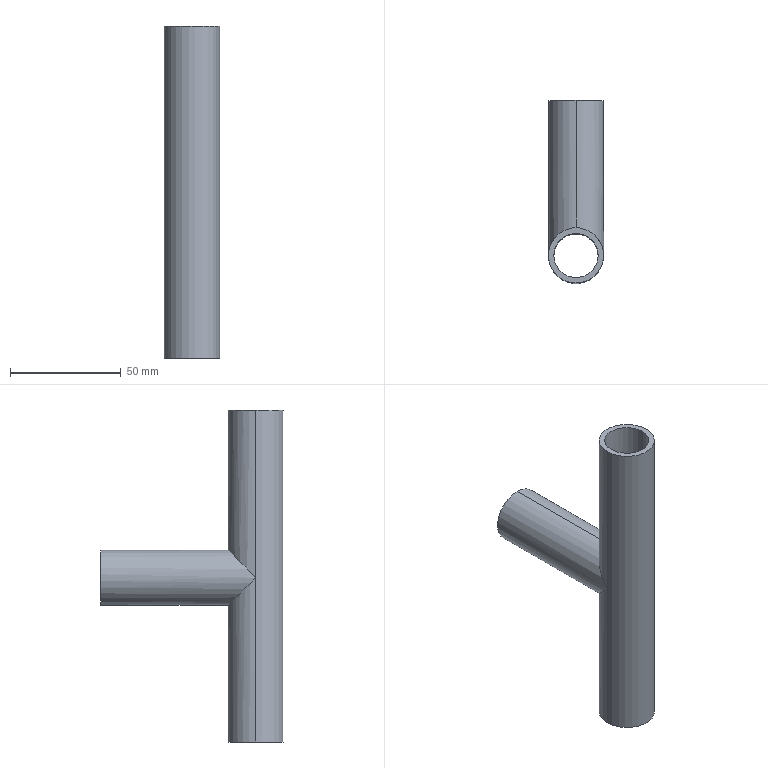Part | SolidWorks | features ICE 2, BaseBody 1 | 1 solid | 17 faces | box 25 x 82.626 x 150 mm | volume 36350 mm3 | cylinder 12 | plane 5 | commonest cylinder face diameters 20 x7 25 x5
STEP:
#1=CARTESIAN_POINT('',(0.,10.,64.222));
#2=VERTEX_POINT('',#1);
#3=CARTESIAN_POINT('',(-10.,0.,74.222));
#4=VERTEX_POINT('',#3);
#5=CARTESIAN_POINT('',(0.,10.,64.222));
#6=CARTESIAN_POINT('',(-5.858,10.,64.222));
#7=CARTESIAN_POINT('',(-10.,5.858,68.365));
#8=CARTESIAN_POINT('',(-10.,0.,74.222));
#9=(BOUNDED_CURVE()B_SPLINE_CURVE(3,(#5,#6,#7,#8),.UNSPECIFIED.,.F.,.F.)B_SPLINE_CURVE_WITH_KNOTS((4,4),(0.,1.571),.UNSPECIFIED.)CURVE()GEOMETRIC_REPRESENTATION_ITEM()RATIONAL_B_SPLINE_CURVE((1.,0.8047,0.8047,1.))REPRESENTATION_ITEM(''));
#10=EDGE_CURVE('',#2,#4,#9,.T.);
#11=ORIENTED_EDGE('',*,*,#10,.F.);
#12=CARTESIAN_POINT('',(0.,70.126,64.222));
#13=VERTEX_POINT('',#12);
#14=CARTESIAN_POINT('',(0.,-3.874,64.222));
#15=DIRECTION('',(0.,1.,0.));
#16=VECTOR('',#15,1000.);
#17=LINE('',#14,#16);
#18=EDGE_CURVE('',#2,#13,#17,.T.);
#19=ORIENTED_EDGE('',*,*,#18,.T.);
#20=CARTESIAN_POINT('',(0.,70.126,84.222));
#21=VERTEX_POINT('',#20);
#22=CARTESIAN_POINT('',(0.,70.126,74.222));
#23=DIRECTION('',(0.,1.,0.));
#24=DIRECTION('',(0.,0.,1.));
#25=AXIS2_PLACEMENT_3D('',#22,#23,#24);
#26=CIRCLE('',#25,10.);
#27=EDGE_CURVE('',#13,#21,#26,.T.);
#28=ORIENTED_EDGE('',*,*,#27,.T.);
#29=CARTESIAN_POINT('',(0.,10.,84.222));
#30=VERTEX_POINT('',#29);
#31=CARTESIAN_POINT('',(0.,-3.874,84.222));
#32=DIRECTION('',(0.,1.,0.));
#33=VECTOR('',#32,1000.);
#34=LINE('',#31,#33);
#35=EDGE_CURVE('',#30,#21,#34,.T.);
#36=ORIENTED_EDGE('',*,*,#35,.F.);
#37=CARTESIAN_POINT('',(-10.,0.,74.222));
#38=CARTESIAN_POINT('',(-10.,5.858,80.08));
#39=CARTESIAN_POINT('',(-5.858,10.,84.222));
#40=CARTESIAN_POINT('',(0.,10.,84.222));
#41=(BOUNDED_CURVE()B_SPLINE_CURVE(3,(#37,#38,#39,#40),.UNSPECIFIED.,.F.,.F.)B_SPLINE_CURVE_WITH_KNOTS((4,4),(1.571,3.142),.UNSPECIFIED.)CURVE()GEOMETRIC_REPRESENTATION_ITEM()RATIONAL_B_SPLINE_CURVE((1.,0.8047,0.8047,1.))REPRESENTATION_ITEM(''));
#42=EDGE_CURVE('',#4,#30,#41,.T.);
#43=ORIENTED_EDGE('',*,*,#42,.F.);
#44=EDGE_LOOP('',(#11,#19,#28,#36,#43));
#45=FACE_OUTER_BOUND('',#44,.T.);
#46=CARTESIAN_POINT('',(0.,-3.874,74.222));
#47=DIRECTION('',(0.,1.,0.));
#48=DIRECTION('',(0.,0.,1.));
#49=AXIS2_PLACEMENT_3D('',#46,#47,#48);
#50=CYLINDRICAL_SURFACE('',#49,10.);
#51=ADVANCED_FACE('',(#45),#50,.F.);
#52=CARTESIAN_POINT('',(0.,70.126,86.722));
#53=VERTEX_POINT('',#52);
#54=CARTESIAN_POINT('',(0.,70.126,61.722));
#55=VERTEX_POINT('',#54);
#56=CARTESIAN_POINT('',(0.,70.126,74.222));
#57=DIRECTION('',(0.,1.,0.));
#58=DIRECTION('',(0.,0.,-1.));
#59=AXIS2_PLACEMENT_3D('',#56,#57,#58);
#60=CIRCLE('',#59,12.5);
#61=EDGE_CURVE('',#53,#55,#60,.T.);
#62=ORIENTED_EDGE('',*,*,#61,.F.);
#63=CARTESIAN_POINT('',(0.,12.5,86.722));
#64=VERTEX_POINT('',#63);
#65=CARTESIAN_POINT('',(0.,800.,86.722));
#66=DIRECTION('',(0.,-1.,0.));
#67=VECTOR('',#66,1000.);
#68=LINE('',#65,#67);
#69=EDGE_CURVE('',#53,#64,#68,.T.);
#70=ORIENTED_EDGE('',*,*,#69,.T.);
#71=CARTESIAN_POINT('',(12.5,0.,74.222));
#72=VERTEX_POINT('',#71);
#73=CARTESIAN_POINT('',(0.,12.5,86.722));
#74=CARTESIAN_POINT('',(7.322,12.5,86.722));
#75=CARTESIAN_POINT('',(12.5,7.322,81.545));
#76=CARTESIAN_POINT('',(12.5,0.,74.222));
#77=(BOUNDED_CURVE()B_SPLINE_CURVE(3,(#73,#74,#75,#76),.UNSPECIFIED.,.F.,.F.)B_SPLINE_CURVE_WITH_KNOTS((4,4),(3.142,4.712),.UNSPECIFIED.)CURVE()GEOMETRIC_REPRESENTATION_ITEM()RATIONAL_B_SPLINE_CURVE((1.,0.8047,0.8047,1.))REPRESENTATION_ITEM(''));
#78=EDGE_CURVE('',#64,#72,#77,.T.);
#79=ORIENTED_EDGE('',*,*,#78,.T.);
#80=CARTESIAN_POINT('',(0.,12.5,61.722));
#81=VERTEX_POINT('',#80);
#82=CARTESIAN_POINT('',(12.5,0.,74.222));
#83=CARTESIAN_POINT('',(12.5,7.322,66.9));
#84=CARTESIAN_POINT('',(7.322,12.5,61.722));
#85=CARTESIAN_POINT('',(0.,12.5,61.722));
#86=(BOUNDED_CURVE()B_SPLINE_CURVE(3,(#82,#83,#84,#85),.UNSPECIFIED.,.F.,.F.)B_SPLINE_CURVE_WITH_KNOTS((4,4),(1.571,3.142),.UNSPECIFIED.)CURVE()GEOMETRIC_REPRESENTATION_ITEM()RATIONAL_B_SPLINE_CURVE((1.,0.8047,0.8047,1.))REPRESENTATION_ITEM(''));
#87=EDGE_CURVE('',#72,#81,#86,.T.);
#88=ORIENTED_EDGE('',*,*,#87,.T.);
#89=CARTESIAN_POINT('',(0.,800.,61.722));
#90=DIRECTION('',(0.,-1.,0.));
#91=VECTOR('',#90,1000.);
#92=LINE('',#89,#91);
#93=EDGE_CURVE('',#55,#81,#92,.T.);
#94=ORIENTED_EDGE('',*,*,#93,.F.);
#95=EDGE_LOOP('',(#62,#70,#79,#88,#94));
#96=FACE_OUTER_BOUND('',#95,.T.);
#97=CARTESIAN_POINT('',(0.,800.,74.222));
#98=DIRECTION('',(0.,-1.,0.));
#99=DIRECTION('',(0.,0.,-1.));
#100=AXIS2_PLACEMENT_3D('',#97,#98,#99);
#101=CYLINDRICAL_SURFACE('',#100,12.5);
#102=ADVANCED_FACE('',(#96),#101,.T.);
#103=CARTESIAN_POINT('',(-12.5,0.,150.));
#104=VERTEX_POINT('',#103);
#105=CARTESIAN_POINT('',(12.5,0.,150.));
#106=VERTEX_POINT('',#105);
#107=CARTESIAN_POINT('',(0.,0.,150.));
#108=DIRECTION('',(0.,0.,-1.));
#109=DIRECTION('',(-1.,0.,0.));
#110=AXIS2_PLACEMENT_3D('',#107,#108,#109);
#111=CIRCLE('',#110,12.5);
#112=EDGE_CURVE('',#104,#106,#111,.T.);
#113=ORIENTED_EDGE('',*,*,#112,.T.);
#114=CARTESIAN_POINT('',(12.5,0.,150.));
#115=DIRECTION('',(0.,0.,-1.));
#116=VECTOR('',#115,1000.);
#117=LINE('',#114,#116);
#118=EDGE_CURVE('',#106,#72,#117,.T.);
#119=ORIENTED_EDGE('',*,*,#118,.T.);
#120=ORIENTED_EDGE('',*,*,#78,.F.);
#121=CARTESIAN_POINT('',(-12.5,0.,74.222));
#122=VERTEX_POINT('',#121);
#123=CARTESIAN_POINT('',(-12.5,0.,74.222));
#124=CARTESIAN_POINT('',(-12.5,7.322,81.545));
#125=CARTESIAN_POINT('',(-7.322,12.5,86.722));
#126=CARTESIAN_POINT('',(0.,12.5,86.722));
#127=(BOUNDED_CURVE()B_SPLINE_CURVE(3,(#123,#124,#125,#126),.UNSPECIFIED.,.F.,.F.)B_SPLINE_CURVE_WITH_KNOTS((4,4),(1.571,3.142),.UNSPECIFIED.)CURVE()GEOMETRIC_REPRESENTATION_ITEM()RATIONAL_B_SPLINE_CURVE((1.,0.8047,0.8047,1.))REPRESENTATION_ITEM(''));
#128=EDGE_CURVE('',#122,#64,#127,.T.);
#129=ORIENTED_EDGE('',*,*,#128,.F.);
#130=CARTESIAN_POINT('',(-12.5,0.,150.));
#131=DIRECTION('',(0.,0.,-1.));
#132=VECTOR('',#131,1000.);
#133=LINE('',#130,#132);
#134=EDGE_CURVE('',#104,#122,#133,.T.);
#135=ORIENTED_EDGE('',*,*,#134,.F.);
#136=EDGE_LOOP('',(#113,#119,#120,#129,#135));
#137=FACE_OUTER_BOUND('',#136,.T.);
#138=CARTESIAN_POINT('',(0.,0.,150.));
#139=DIRECTION('',(0.,0.,-1.));
#140=DIRECTION('',(-1.,0.,0.));
#141=AXIS2_PLACEMENT_3D('',#138,#139,#140);
#142=CYLINDRICAL_SURFACE('',#141,12.5);
#143=ADVANCED_FACE('',(#137),#142,.T.);
#144=ORIENTED_EDGE('',*,*,#87,.F.);
#145=CARTESIAN_POINT('',(12.5,0.,0.));
#146=VERTEX_POINT('',#145);
#147=CARTESIAN_POINT('',(12.5,0.,150.));
#148=DIRECTION('',(0.,0.,-1.));
#149=VECTOR('',#148,1000.);
#150=LINE('',#147,#149);
#151=EDGE_CURVE('',#72,#146,#150,.T.);
#152=ORIENTED_EDGE('',*,*,#151,.T.);
#153=CARTESIAN_POINT('',(-12.5,0.,0.));
#154=VERTEX_POINT('',#153);
#155=CARTESIAN_POINT('',(0.,0.,0.));
#156=DIRECTION('',(0.,0.,1.));
#157=DIRECTION('',(-1.,0.,0.));
#158=AXIS2_PLACEMENT_3D('',#155,#156,#157);
#159=CIRCLE('',#158,12.5);
#160=EDGE_CURVE('',#146,#154,#159,.T.);
#161=ORIENTED_EDGE('',*,*,#160,.T.);
#162=CARTESIAN_POINT('',(-12.5,0.,150.));
#163=DIRECTION('',(0.,0.,-1.));
#164=VECTOR('',#163,1000.);
#165=LINE('',#162,#164);
#166=EDGE_CURVE('',#122,#154,#165,.T.);
#167=ORIENTED_EDGE('',*,*,#166,.F.);
#168=CARTESIAN_POINT('',(0.,12.5,61.722));
#169=CARTESIAN_POINT('',(-7.322,12.5,61.722));
#170=CARTESIAN_POINT('',(-12.5,7.322,66.9));
#171=CARTESIAN_POINT('',(-12.5,0.,74.222));
#172=(BOUNDED_CURVE()B_SPLINE_CURVE(3,(#168,#169,#170,#171),.UNSPECIFIED.,.F.,.F.)B_SPLINE_CURVE_WITH_KNOTS((4,4),(3.142,4.712),.UNSPECIFIED.)CURVE()GEOMETRIC_REPRESENTATION_ITEM()RATIONAL_B_SPLINE_CURVE((1.,0.8047,0.8047,1.))REPRESENTATION_ITEM(''));
#173=EDGE_CURVE('',#81,#122,#172,.T.);
#174=ORIENTED_EDGE('',*,*,#173,.F.);
#175=EDGE_LOOP('',(#144,#152,#161,#167,#174));
#176=FACE_OUTER_BOUND('',#175,.T.);
#177=CARTESIAN_POINT('',(0.,0.,150.));
#178=DIRECTION('',(0.,0.,-1.));
#179=DIRECTION('',(-1.,0.,0.));
#180=AXIS2_PLACEMENT_3D('',#177,#178,#179);
#181=CYLINDRICAL_SURFACE('',#180,12.5);
#182=ADVANCED_FACE('',(#176),#181,.T.);
#183=CARTESIAN_POINT('',(10.,0.,150.));
#184=VERTEX_POINT('',#183);
#185=CARTESIAN_POINT('',(-10.,0.,150.));
#186=VERTEX_POINT('',#185);
#187=CARTESIAN_POINT('',(0.,0.,150.));
#188=DIRECTION('',(0.,0.,-1.));
#189=DIRECTION('',(-1.,0.,0.));
#190=AXIS2_PLACEMENT_3D('',#187,#188,#189);
#191=CIRCLE('',#190,10.);
#192=EDGE_CURVE('',#184,#186,#191,.T.);
#193=ORIENTED_EDGE('',*,*,#192,.F.);
#194=CARTESIAN_POINT('',(10.,0.,74.222));
#195=VERTEX_POINT('',#194);
#196=CARTESIAN_POINT('',(10.,0.,150.));
#197=DIRECTION('',(0.,0.,-1.));
#198=VECTOR('',#197,1000.);
#199=LINE('',#196,#198);
#200=EDGE_CURVE('',#184,#195,#199,.T.);
#201=ORIENTED_EDGE('',*,*,#200,.T.);
#202=CARTESIAN_POINT('',(9.219,-3.874,78.097));
#203=VERTEX_POINT('',#202);
#204=CARTESIAN_POINT('',(10.,0.,74.222));
#205=CARTESIAN_POINT('',(10.,-1.335,75.557));
#206=CARTESIAN_POINT('',(9.736,-2.644,76.866));
#207=CARTESIAN_POINT('',(9.219,-3.874,78.097));
#208=(BOUNDED_CURVE()B_SPLINE_CURVE(3,(#204,#205,#206,#207),.UNSPECIFIED.,.F.,.F.)B_SPLINE_CURVE_WITH_KNOTS((4,4),(1.571,1.969),.UNSPECIFIED.)CURVE()GEOMETRIC_REPRESENTATION_ITEM()RATIONAL_B_SPLINE_CURVE((1.,0.9869,0.9869,1.))REPRESENTATION_ITEM(''));
#209=EDGE_CURVE('',#195,#203,#208,.T.);
#210=ORIENTED_EDGE('',*,*,#209,.T.);
#211=CARTESIAN_POINT('',(9.219,-3.874,70.348));
#212=VERTEX_POINT('',#211);
#213=CARTESIAN_POINT('',(9.219,-3.874,150.));
#214=DIRECTION('',(0.,0.,1.));
#215=VECTOR('',#214,1000.);
#216=LINE('',#213,#215);
#217=EDGE_CURVE('',#212,#203,#216,.T.);
#218=ORIENTED_EDGE('',*,*,#217,.F.);
#219=CARTESIAN_POINT('',(9.219,-3.874,70.348));
#220=CARTESIAN_POINT('',(9.736,-2.644,71.579));
#221=CARTESIAN_POINT('',(10.,-1.335,72.887));
#222=CARTESIAN_POINT('',(10.,0.,74.222));
#223=(BOUNDED_CURVE()B_SPLINE_CURVE(3,(#219,#220,#221,#222),.UNSPECIFIED.,.F.,.F.)B_SPLINE_CURVE_WITH_KNOTS((4,4),(1.173,1.571),.UNSPECIFIED.)CURVE()GEOMETRIC_REPRESENTATION_ITEM()RATIONAL_B_SPLINE_CURVE((1.,0.9869,0.9869,1.))REPRESENTATION_ITEM(''));
#224=EDGE_CURVE('',#212,#195,#223,.T.);
#225=ORIENTED_EDGE('',*,*,#224,.T.);
#226=CARTESIAN_POINT('',(10.,0.,0.));
#227=VERTEX_POINT('',#226);
#228=CARTESIAN_POINT('',(10.,0.,150.));
#229=DIRECTION('',(0.,0.,-1.));
#230=VECTOR('',#229,1000.);
#231=LINE('',#228,#230);
#232=EDGE_CURVE('',#195,#227,#231,.T.);
#233=ORIENTED_EDGE('',*,*,#232,.T.);
#234=CARTESIAN_POINT('',(-10.,0.,0.));
#235=VERTEX_POINT('',#234);
#236=CARTESIAN_POINT('',(0.,0.,0.));
#237=DIRECTION('',(0.,0.,-1.));
#238=DIRECTION('',(-1.,0.,0.));
#239=AXIS2_PLACEMENT_3D('',#236,#237,#238);
#240=CIRCLE('',#239,10.);
#241=EDGE_CURVE('',#227,#235,#240,.T.);
#242=ORIENTED_EDGE('',*,*,#241,.T.);
#243=CARTESIAN_POINT('',(-10.,0.,150.));
#244=DIRECTION('',(0.,0.,-1.));
#245=VECTOR('',#244,1000.);
#246=LINE('',#243,#245);
#247=EDGE_CURVE('',#4,#235,#246,.T.);
#248=ORIENTED_EDGE('',*,*,#247,.F.);
#249=CARTESIAN_POINT('',(-9.219,-3.874,70.348));
#250=VERTEX_POINT('',#249);
#251=CARTESIAN_POINT('',(-10.,0.,74.222));
#252=CARTESIAN_POINT('',(-10.,-1.335,72.887));
#253=CARTESIAN_POINT('',(-9.736,-2.644,71.579));
#254=CARTESIAN_POINT('',(-9.219,-3.874,70.348));
#255=(BOUNDED_CURVE()B_SPLINE_CURVE(3,(#251,#252,#253,#254),.UNSPECIFIED.,.F.,.F.)B_SPLINE_CURVE_WITH_KNOTS((4,4),(4.712,5.11),.UNSPECIFIED.)CURVE()GEOMETRIC_REPRESENTATION_ITEM()RATIONAL_B_SPLINE_CURVE((1.,0.9869,0.9869,1.))REPRESENTATION_ITEM(''));
#256=EDGE_CURVE('',#4,#250,#255,.T.);
#257=ORIENTED_EDGE('',*,*,#256,.T.);
#258=CARTESIAN_POINT('',(-9.219,-3.874,78.097));
#259=VERTEX_POINT('',#258);
#260=CARTESIAN_POINT('',(-9.219,-3.874,150.));
#261=DIRECTION('',(0.,0.,-1.));
#262=VECTOR('',#261,1000.);
#263=LINE('',#260,#262);
#264=EDGE_CURVE('',#259,#250,#263,.T.);
#265=ORIENTED_EDGE('',*,*,#264,.F.);
#266=CARTESIAN_POINT('',(-9.219,-3.874,78.097));
#267=CARTESIAN_POINT('',(-9.736,-2.644,76.866));
#268=CARTESIAN_POINT('',(-10.,-1.335,75.557));
#269=CARTESIAN_POINT('',(-10.,0.,74.222));
#270=(BOUNDED_CURVE()B_SPLINE_CURVE(3,(#266,#267,#268,#269),.UNSPECIFIED.,.F.,.F.)B_SPLINE_CURVE_WITH_KNOTS((4,4),(4.315,4.712),.UNSPECIFIED.)CURVE()GEOMETRIC_REPRESENTATION_ITEM()RATIONAL_B_SPLINE_CURVE((1.,0.9869,0.9869,1.))REPRESENTATION_ITEM(''));
#271=EDGE_CURVE('',#259,#4,#270,.T.);
#272=ORIENTED_EDGE('',*,*,#271,.T.);
#273=CARTESIAN_POINT('',(-10.,0.,150.));
#274=DIRECTION('',(0.,0.,-1.));
#275=VECTOR('',#274,1000.);
#276=LINE('',#273,#275);
#277=EDGE_CURVE('',#186,#4,#276,.T.);
#278=ORIENTED_EDGE('',*,*,#277,.F.);
#279=EDGE_LOOP('',(#193,#201,#210,#218,#225,#233,#242,#248,#257,#265,#272,#278));
#280=FACE_OUTER_BOUND('',#279,.T.);
#281=CARTESIAN_POINT('',(0.,0.,150.));
#282=DIRECTION('',(0.,0.,-1.));
#283=DIRECTION('',(-1.,0.,0.));
#284=AXIS2_PLACEMENT_3D('',#281,#282,#283);
#285=CYLINDRICAL_SURFACE('',#284,10.);
#286=ADVANCED_FACE('',(#280),#285,.F.);
#287=ORIENTED_EDGE('',*,*,#200,.F.);
#288=CARTESIAN_POINT('',(0.,0.,150.));
#289=DIRECTION('',(0.,0.,-1.));
#290=DIRECTION('',(-1.,0.,0.));
#291=AXIS2_PLACEMENT_3D('',#288,#289,#290);
#292=CIRCLE('',#291,10.);
#293=EDGE_CURVE('',#186,#184,#292,.T.);
#294=ORIENTED_EDGE('',*,*,#293,.F.);
#295=ORIENTED_EDGE('',*,*,#277,.T.);
#296=ORIENTED_EDGE('',*,*,#42,.T.);
#297=CARTESIAN_POINT('',(0.,10.,84.222));
#298=CARTESIAN_POINT('',(5.858,10.,84.222));
#299=CARTESIAN_POINT('',(10.,5.858,80.08));
#300=CARTESIAN_POINT('',(10.,0.,74.222));
#301=(BOUNDED_CURVE()B_SPLINE_CURVE(3,(#297,#298,#299,#300),.UNSPECIFIED.,.F.,.F.)B_SPLINE_CURVE_WITH_KNOTS((4,4),(3.142,4.712),.UNSPECIFIED.)CURVE()GEOMETRIC_REPRESENTATION_ITEM()RATIONAL_B_SPLINE_CURVE((1.,0.8047,0.8047,1.))REPRESENTATION_ITEM(''));
#302=EDGE_CURVE('',#30,#195,#301,.T.);
#303=ORIENTED_EDGE('',*,*,#302,.T.);
#304=EDGE_LOOP('',(#287,#294,#295,#296,#303));
#305=FACE_OUTER_BOUND('',#304,.T.);
#306=CARTESIAN_POINT('',(0.,0.,150.));
#307=DIRECTION('',(0.,0.,-1.));
#308=DIRECTION('',(-1.,0.,0.));
#309=AXIS2_PLACEMENT_3D('',#306,#307,#308);
#310=CYLINDRICAL_SURFACE('',#309,10.);
#311=ADVANCED_FACE('',(#305),#310,.F.);
#312=ORIENTED_EDGE('',*,*,#69,.F.);
#313=CARTESIAN_POINT('',(0.,70.126,74.222));
#314=DIRECTION('',(0.,1.,0.));
#315=DIRECTION('',(0.,0.,-1.));
#316=AXIS2_PLACEMENT_3D('',#313,#314,#315);
#317=CIRCLE('',#316,12.5);
#318=EDGE_CURVE('',#55,#53,#317,.T.);
#319=ORIENTED_EDGE('',*,*,#318,.F.);
#320=ORIENTED_EDGE('',*,*,#93,.T.);
#321=ORIENTED_EDGE('',*,*,#173,.T.);
#322=ORIENTED_EDGE('',*,*,#128,.T.);
#323=EDGE_LOOP('',(#312,#319,#320,#321,#322));
#324=FACE_OUTER_BOUND('',#323,.T.);
#325=CARTESIAN_POINT('',(0.,800.,74.222));
#326=DIRECTION('',(0.,-1.,0.));
#327=DIRECTION('',(0.,0.,-1.));
#328=AXIS2_PLACEMENT_3D('',#325,#326,#327);
#329=CYLINDRICAL_SURFACE('',#328,12.5);
#330=ADVANCED_FACE('',(#324),#329,.T.);
#331=ORIENTED_EDGE('',*,*,#118,.F.);
#332=CARTESIAN_POINT('',(0.,0.,150.));
#333=DIRECTION('',(0.,0.,-1.));
#334=DIRECTION('',(-1.,0.,0.));
#335=AXIS2_PLACEMENT_3D('',#332,#333,#334);
#336=CIRCLE('',#335,12.5);
#337=EDGE_CURVE('',#106,#104,#336,.T.);
#338=ORIENTED_EDGE('',*,*,#337,.T.);
#339=ORIENTED_EDGE('',*,*,#134,.T.);
#340=ORIENTED_EDGE('',*,*,#166,.T.);
#341=CARTESIAN_POINT('',(0.,0.,0.));
#342=DIRECTION('',(0.,0.,1.));
#343=DIRECTION('',(-1.,0.,0.));
#344=AXIS2_PLACEMENT_3D('',#341,#342,#343);
#345=CIRCLE('',#344,12.5);
#346=EDGE_CURVE('',#154,#146,#345,.T.);
#347=ORIENTED_EDGE('',*,*,#346,.T.);
#348=ORIENTED_EDGE('',*,*,#151,.F.);
#349=EDGE_LOOP('',(#331,#338,#339,#340,#347,#348));
#350=FACE_OUTER_BOUND('',#349,.T.);
#351=CARTESIAN_POINT('',(0.,0.,150.));
#352=DIRECTION('',(0.,0.,-1.));
#353=DIRECTION('',(-1.,0.,0.));
#354=AXIS2_PLACEMENT_3D('',#351,#352,#353);
#355=CYLINDRICAL_SURFACE('',#354,12.5);
#356=ADVANCED_FACE('',(#350),#355,.T.);
#357=CARTESIAN_POINT('',(0.,0.,0.));
#358=DIRECTION('',(0.,0.,-1.));
#359=DIRECTION('',(-1.,0.,0.));
#360=AXIS2_PLACEMENT_3D('',#357,#358,#359);
#361=CIRCLE('',#360,10.);
#362=EDGE_CURVE('',#235,#227,#361,.T.);
#363=ORIENTED_EDGE('',*,*,#362,.F.);
#364=ORIENTED_EDGE('',*,*,#241,.F.);
#365=EDGE_LOOP('',(#363,#364));
#366=FACE_BOUND('',#365,.T.);
#367=ORIENTED_EDGE('',*,*,#346,.F.);
#368=ORIENTED_EDGE('',*,*,#160,.F.);
#369=EDGE_LOOP('',(#367,#368));
#370=FACE_OUTER_BOUND('',#369,.T.);
#371=CARTESIAN_POINT('',(0.,0.,0.));
#372=DIRECTION('',(0.,0.,1.));
#373=DIRECTION('',(1.,0.,0.));
#374=AXIS2_PLACEMENT_3D('',#371,#372,#373);
#375=PLANE('',#374);
#376=ADVANCED_FACE('',(#366,#370),#375,.F.);
#377=ORIENTED_EDGE('',*,*,#293,.T.);
#378=ORIENTED_EDGE('',*,*,#192,.T.);
#379=EDGE_LOOP('',(#377,#378));
#380=FACE_BOUND('',#379,.T.);
#381=ORIENTED_EDGE('',*,*,#112,.F.);
#382=ORIENTED_EDGE('',*,*,#337,.F.);
#383=EDGE_LOOP('',(#381,#382));
#384=FACE_OUTER_BOUND('',#383,.T.);
#385=CARTESIAN_POINT('',(0.,0.,150.));
#386=DIRECTION('',(0.,0.,1.));
#387=DIRECTION('',(1.,0.,0.));
#388=AXIS2_PLACEMENT_3D('',#385,#386,#387);
#389=PLANE('',#388);
#390=ADVANCED_FACE('',(#380,#384),#389,.T.);
#391=ORIENTED_EDGE('',*,*,#232,.F.);
#392=CARTESIAN_POINT('',(10.,0.,74.222));
#393=CARTESIAN_POINT('',(10.,5.858,68.365));
#394=CARTESIAN_POINT('',(5.858,10.,64.222));
#395=CARTESIAN_POINT('',(0.,10.,64.222));
#396=(BOUNDED_CURVE()B_SPLINE_CURVE(3,(#392,#393,#394,#395),.UNSPECIFIED.,.F.,.F.)B_SPLINE_CURVE_WITH_KNOTS((4,4),(4.712,6.283),.UNSPECIFIED.)CURVE()GEOMETRIC_REPRESENTATION_ITEM()RATIONAL_B_SPLINE_CURVE((1.,0.8047,0.8047,1.))REPRESENTATION_ITEM(''));
#397=EDGE_CURVE('',#195,#2,#396,.T.);
#398=ORIENTED_EDGE('',*,*,#397,.T.);
#399=ORIENTED_EDGE('',*,*,#10,.T.);
#400=ORIENTED_EDGE('',*,*,#247,.T.);
#401=ORIENTED_EDGE('',*,*,#362,.T.);
#402=EDGE_LOOP('',(#391,#398,#399,#400,#401));
#403=FACE_OUTER_BOUND('',#402,.T.);
#404=CARTESIAN_POINT('',(0.,0.,150.));
#405=DIRECTION('',(0.,0.,-1.));
#406=DIRECTION('',(-1.,0.,0.));
#407=AXIS2_PLACEMENT_3D('',#404,#405,#406);
#408=CYLINDRICAL_SURFACE('',#407,10.);
#409=ADVANCED_FACE('',(#403),#408,.F.);
#410=CARTESIAN_POINT('',(0.,70.126,74.222));
#411=DIRECTION('',(0.,1.,0.));
#412=DIRECTION('',(0.,0.,1.));
#413=AXIS2_PLACEMENT_3D('',#410,#411,#412);
#414=CIRCLE('',#413,10.);
#415=EDGE_CURVE('',#21,#13,#414,.T.);
#416=ORIENTED_EDGE('',*,*,#415,.F.);
#417=ORIENTED_EDGE('',*,*,#27,.F.);
#418=EDGE_LOOP('',(#416,#417));
#419=FACE_BOUND('',#418,.T.);
#420=ORIENTED_EDGE('',*,*,#318,.T.);
#421=ORIENTED_EDGE('',*,*,#61,.T.);
#422=EDGE_LOOP('',(#420,#421));
#423=FACE_OUTER_BOUND('',#422,.T.);
#424=CARTESIAN_POINT('',(-12.5,70.126,317.888));
#425=DIRECTION('',(0.,-1.,0.));
#426=DIRECTION('',(0.,0.,-1.));
#427=AXIS2_PLACEMENT_3D('',#424,#425,#426);
#428=PLANE('',#427);
#429=ADVANCED_FACE('',(#419,#423),#428,.F.);
#430=ORIENTED_EDGE('',*,*,#18,.F.);
#431=ORIENTED_EDGE('',*,*,#397,.F.);
#432=ORIENTED_EDGE('',*,*,#302,.F.);
#433=ORIENTED_EDGE('',*,*,#35,.T.);
#434=ORIENTED_EDGE('',*,*,#415,.T.);
#435=EDGE_LOOP('',(#430,#431,#432,#433,#434));
#436=FACE_OUTER_BOUND('',#435,.T.);
#437=CARTESIAN_POINT('',(0.,-3.874,74.222));
#438=DIRECTION('',(0.,1.,0.));
#439=DIRECTION('',(0.,0.,1.));
#440=AXIS2_PLACEMENT_3D('',#437,#438,#439);
#441=CYLINDRICAL_SURFACE('',#440,10.);
#442=ADVANCED_FACE('',(#436),#441,.F.);
#443=ORIENTED_EDGE('',*,*,#264,.T.);
#444=CARTESIAN_POINT('',(0.,-3.874,74.222));
#445=DIRECTION('',(0.,1.,0.));
#446=DIRECTION('',(0.,0.,1.));
#447=AXIS2_PLACEMENT_3D('',#444,#445,#446);
#448=CIRCLE('',#447,10.);
#449=EDGE_CURVE('',#250,#259,#448,.T.);
#450=ORIENTED_EDGE('',*,*,#449,.T.);
#451=EDGE_LOOP('',(#443,#450));
#452=FACE_OUTER_BOUND('',#451,.T.);
#453=CARTESIAN_POINT('',(0.,-3.874,74.222));
#454=DIRECTION('',(0.,1.,0.));
#455=DIRECTION('',(0.,0.,1.));
#456=AXIS2_PLACEMENT_3D('',#453,#454,#455);
#457=PLANE('',#456);
#458=ADVANCED_FACE('',(#452),#457,.T.);
#459=ORIENTED_EDGE('',*,*,#271,.F.);
#460=ORIENTED_EDGE('',*,*,#449,.F.);
#461=ORIENTED_EDGE('',*,*,#256,.F.);
#462=EDGE_LOOP('',(#459,#460,#461));
#463=FACE_OUTER_BOUND('',#462,.T.);
#464=CARTESIAN_POINT('',(0.,-3.874,74.222));
#465=DIRECTION('',(0.,1.,0.));
#466=DIRECTION('',(0.,0.,1.));
#467=AXIS2_PLACEMENT_3D('',#464,#465,#466);
#468=CYLINDRICAL_SURFACE('',#467,10.);
#469=ADVANCED_FACE('',(#463),#468,.F.);
#470=ORIENTED_EDGE('',*,*,#217,.T.);
#471=CARTESIAN_POINT('',(0.,-3.874,74.222));
#472=DIRECTION('',(0.,1.,0.));
#473=DIRECTION('',(0.,0.,1.));
#474=AXIS2_PLACEMENT_3D('',#471,#472,#473);
#475=CIRCLE('',#474,10.);
#476=EDGE_CURVE('',#203,#212,#475,.T.);
#477=ORIENTED_EDGE('',*,*,#476,.T.);
#478=EDGE_LOOP('',(#470,#477));
#479=FACE_OUTER_BOUND('',#478,.T.);
#480=CARTESIAN_POINT('',(0.,-3.874,74.222));
#481=DIRECTION('',(0.,1.,0.));
#482=DIRECTION('',(0.,0.,1.));
#483=AXIS2_PLACEMENT_3D('',#480,#481,#482);
#484=PLANE('',#483);
#485=ADVANCED_FACE('',(#479),#484,.T.);
#486=ORIENTED_EDGE('',*,*,#476,.F.);
#487=ORIENTED_EDGE('',*,*,#209,.F.);
#488=ORIENTED_EDGE('',*,*,#224,.F.);
#489=EDGE_LOOP('',(#486,#487,#488));
#490=FACE_OUTER_BOUND('',#489,.T.);
#491=CARTESIAN_POINT('',(0.,-3.874,74.222));
#492=DIRECTION('',(0.,1.,0.));
#493=DIRECTION('',(0.,0.,1.));
#494=AXIS2_PLACEMENT_3D('',#491,#492,#493);
#495=CYLINDRICAL_SURFACE('',#494,10.);
#496=ADVANCED_FACE('',(#490),#495,.F.);
#497=CLOSED_SHELL('',(#51,#102,#143,#182,#286,#311,#330,#356,#376,#390,#409,#429,#442,#458,#469,#485,#496));
#498=MANIFOLD_SOLID_BREP('',#497);
#499=CARTESIAN_POINT('',(0.,0.,0.));
#500=DIRECTION('',(0.,0.,1.));
#501=DIRECTION('',(1.,0.,0.));
#502=AXIS2_PLACEMENT_3D('',#499,#500,#501);
#503=(LENGTH_UNIT()NAMED_UNIT(*)SI_UNIT(.MILLI.,.METRE.));
#504=UNCERTAINTY_MEASURE_WITH_UNIT(LENGTH_MEASURE(0.00001),#503,'','');
#505=(NAMED_UNIT(*)PLANE_ANGLE_UNIT()SI_UNIT($,.RADIAN.));
#506=(NAMED_UNIT(*)SI_UNIT($,.STERADIAN.)SOLID_ANGLE_UNIT());
#507=(GEOMETRIC_REPRESENTATION_CONTEXT(3)GLOBAL_UNCERTAINTY_ASSIGNED_CONTEXT((#504))GLOBAL_UNIT_ASSIGNED_CONTEXT((#503,#505,#506))REPRESENTATION_CONTEXT('',''));
#508=ADVANCED_BREP_SHAPE_REPRESENTATION('',(#498,#502),#507);